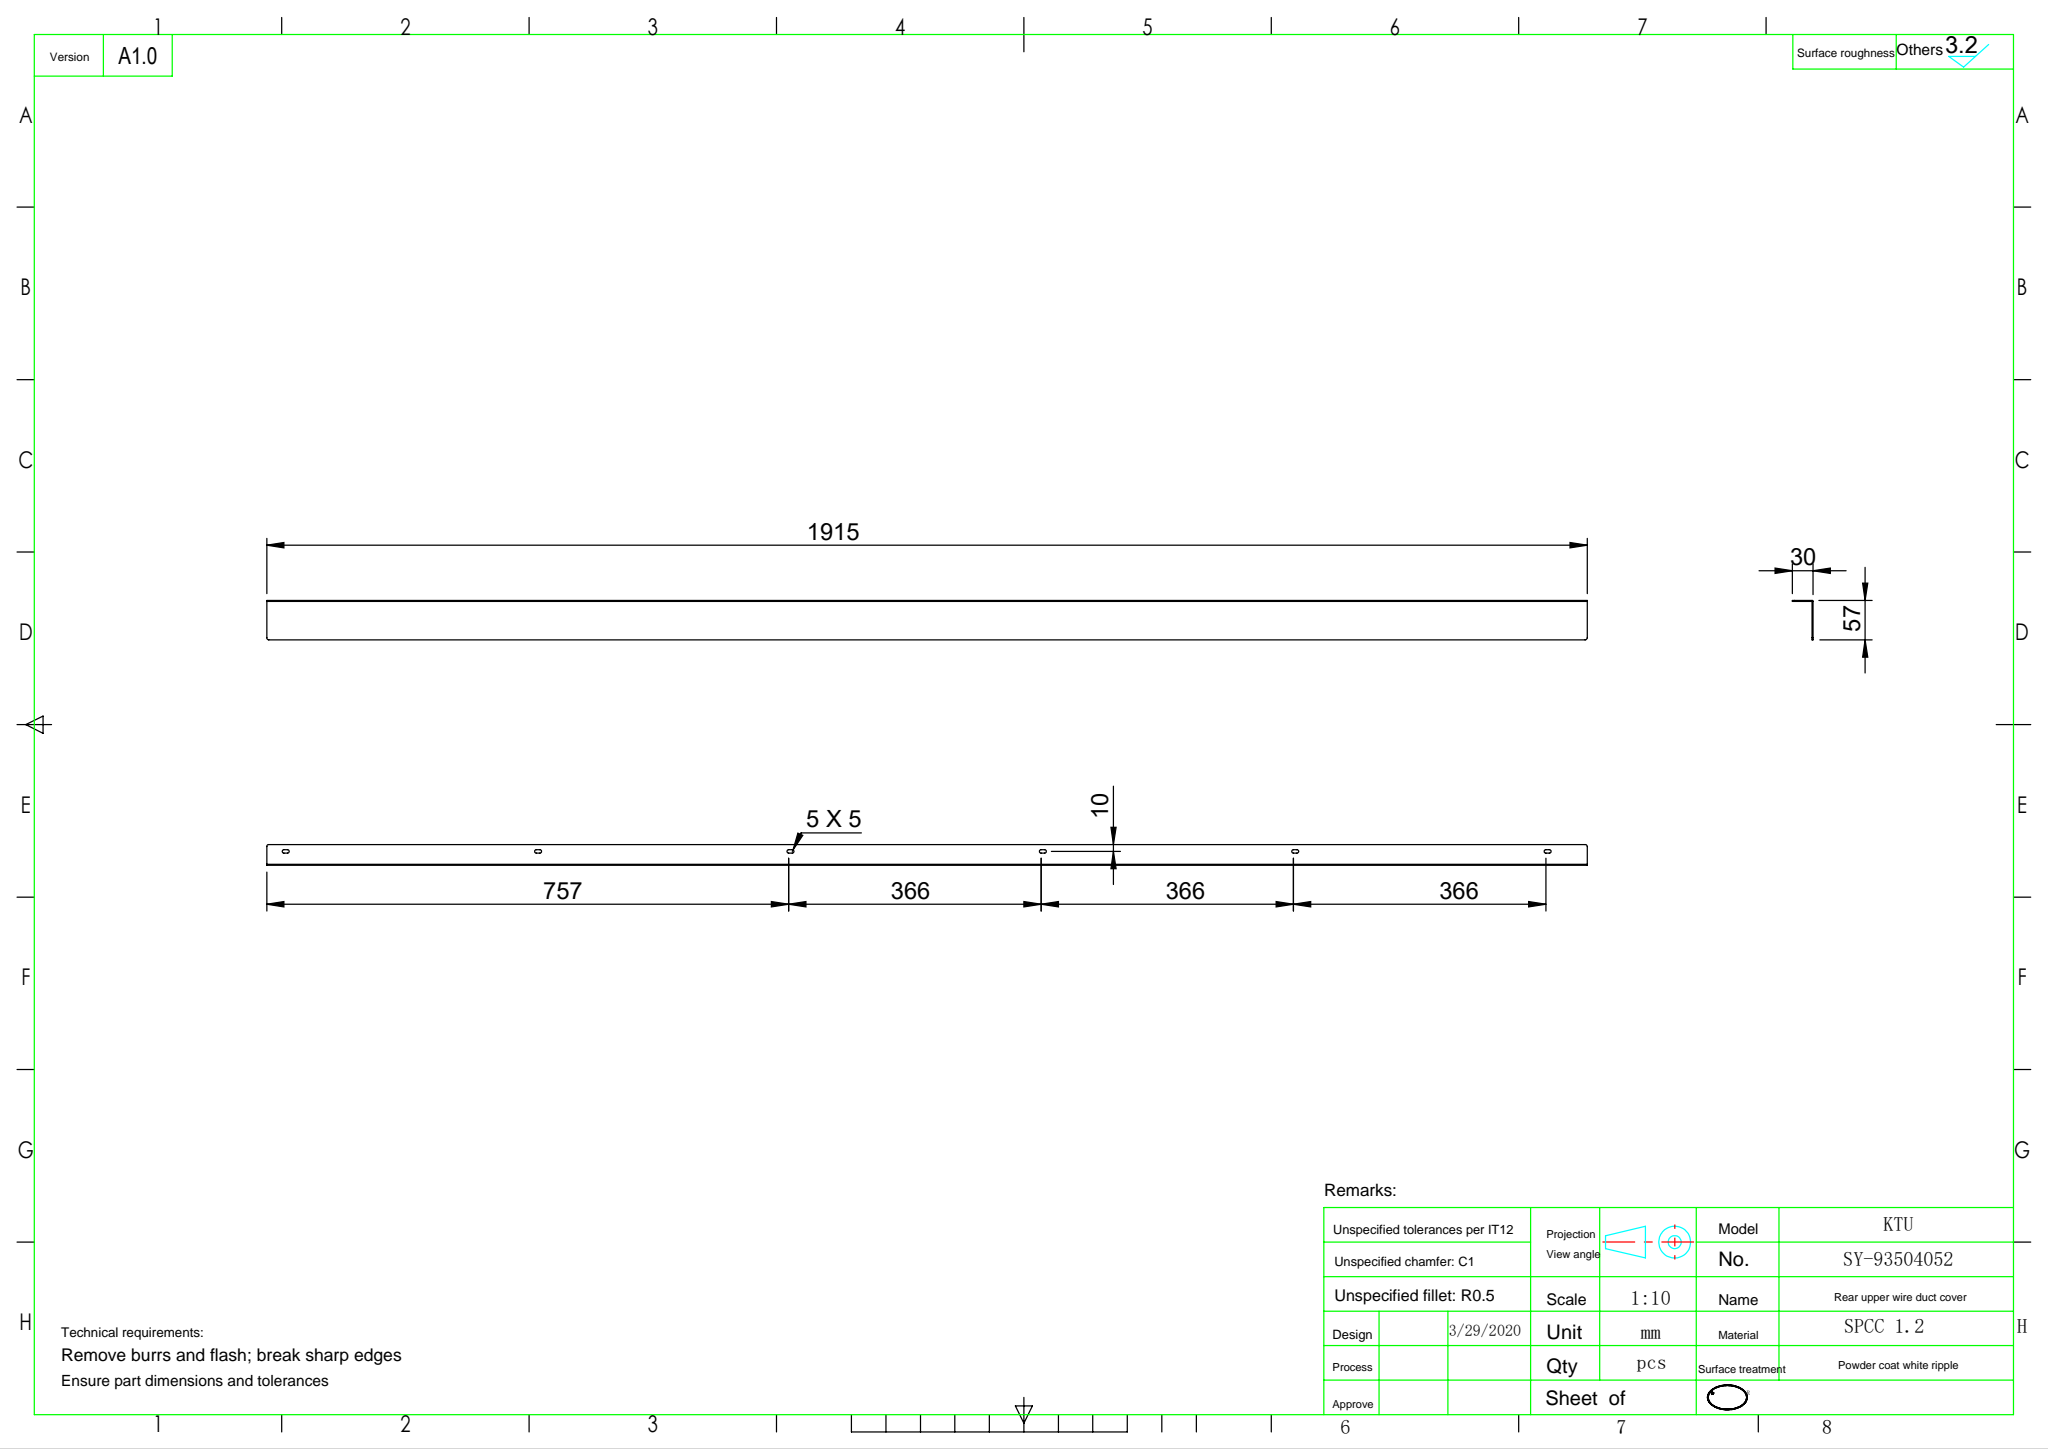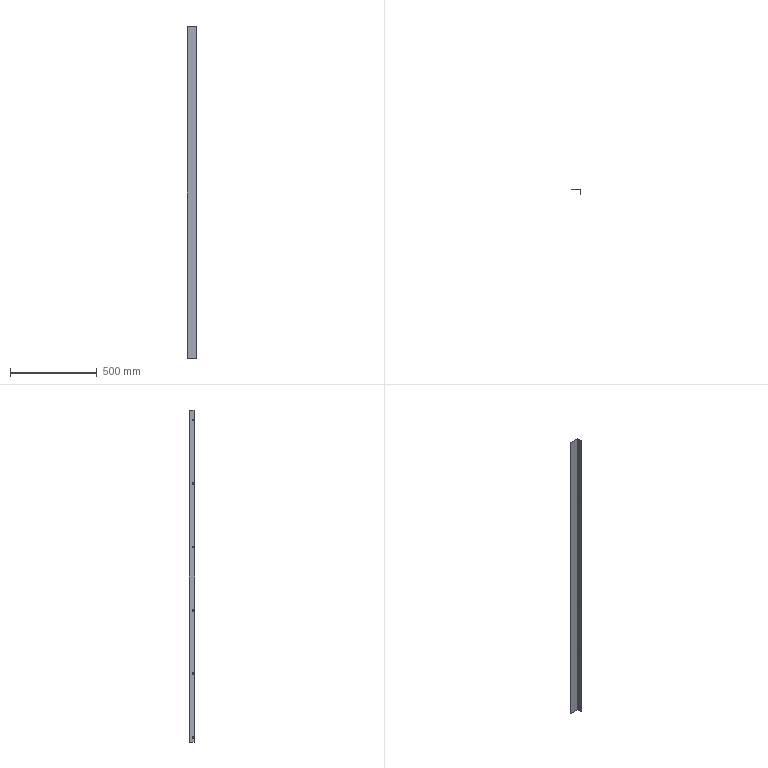Part | SolidWorks | features Fillet 1, FlatPattern 1, ICE 1, LPattern 1, SMBaseFlange 1, SheetMetal 1 | 1 solid | 48 faces | box 57 x 30 x 1915 mm | volume 196049 mm3 | cylinder 24 | plane 24 | commonest cylinder face diameters 5 x18 6 x4 0.4 x1 2.8 x1